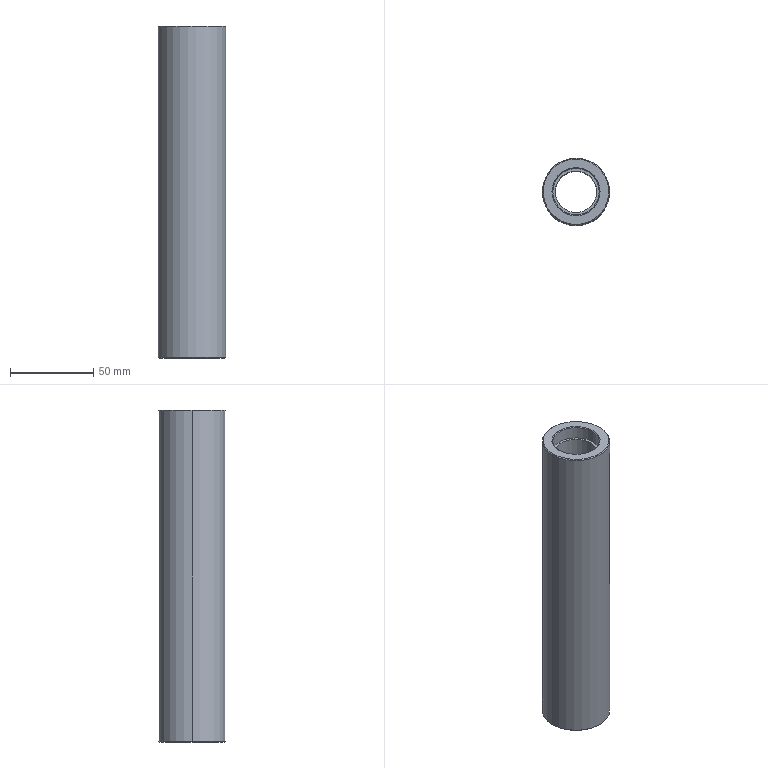Part | SolidWorks | features ICE 2, Chamfer 1, Extrusion 1, MirrorPattern 1 | 1 solid | 20 faces | box 40.5 x 40.5 x 200 mm | volume 157423 mm3 | cone 8 | cylinder 8 | plane 4 | commonest cylinder face diameters 28 x4 25 x2 40.5 x2
STEP:
#1=CARTESIAN_POINT('',(19.75,0.,100.));
#2=VERTEX_POINT('',#1);
#3=CARTESIAN_POINT('',(-19.75,0.,100.));
#4=VERTEX_POINT('',#3);
#5=CARTESIAN_POINT('',(0.,0.,100.));
#6=DIRECTION('',(0.,0.,1.));
#7=DIRECTION('',(1.,0.,0.));
#8=AXIS2_PLACEMENT_3D('',#5,#6,#7);
#9=CIRCLE('',#8,19.75);
#10=EDGE_CURVE('',#2,#4,#9,.T.);
#11=ORIENTED_EDGE('',*,*,#10,.F.);
#12=CARTESIAN_POINT('',(20.25,0.,99.5));
#13=VERTEX_POINT('',#12);
#14=CARTESIAN_POINT('',(19.75,0.,100.));
#15=DIRECTION('',(0.7071,0.,-0.7071));
#16=VECTOR('',#15,1000.);
#17=LINE('',#14,#16);
#18=EDGE_CURVE('',#2,#13,#17,.T.);
#19=ORIENTED_EDGE('',*,*,#18,.T.);
#20=CARTESIAN_POINT('',(-20.25,0.,99.5));
#21=VERTEX_POINT('',#20);
#22=CARTESIAN_POINT('',(0.,0.,99.5));
#23=DIRECTION('',(0.,0.,-1.));
#24=DIRECTION('',(1.,0.,0.));
#25=AXIS2_PLACEMENT_3D('',#22,#23,#24);
#26=CIRCLE('',#25,20.25);
#27=EDGE_CURVE('',#21,#13,#26,.T.);
#28=ORIENTED_EDGE('',*,*,#27,.F.);
#29=CARTESIAN_POINT('',(-19.75,0.,100.));
#30=DIRECTION('',(-0.7071,0.,-0.7071));
#31=VECTOR('',#30,1000.);
#32=LINE('',#29,#31);
#33=EDGE_CURVE('',#4,#21,#32,.T.);
#34=ORIENTED_EDGE('',*,*,#33,.F.);
#35=EDGE_LOOP('',(#11,#19,#28,#34));
#36=FACE_OUTER_BOUND('',#35,.T.);
#37=CARTESIAN_POINT('',(0.,0.,100.));
#38=DIRECTION('',(0.,0.,-1.));
#39=DIRECTION('',(-1.,0.,0.));
#40=AXIS2_PLACEMENT_3D('',#37,#38,#39);
#41=CONICAL_SURFACE('',#40,19.75,0.7854);
#42=ADVANCED_FACE('',(#36),#41,.T.);
#43=CARTESIAN_POINT('',(-19.75,0.,-100.));
#44=VERTEX_POINT('',#43);
#45=CARTESIAN_POINT('',(19.75,0.,-100.));
#46=VERTEX_POINT('',#45);
#47=CARTESIAN_POINT('',(0.,0.,-100.));
#48=DIRECTION('',(0.,0.,-1.));
#49=DIRECTION('',(1.,0.,0.));
#50=AXIS2_PLACEMENT_3D('',#47,#48,#49);
#51=CIRCLE('',#50,19.75);
#52=EDGE_CURVE('',#44,#46,#51,.T.);
#53=ORIENTED_EDGE('',*,*,#52,.F.);
#54=CARTESIAN_POINT('',(-20.25,0.,-99.5));
#55=VERTEX_POINT('',#54);
#56=CARTESIAN_POINT('',(-20.25,0.,-99.5));
#57=DIRECTION('',(-0.7071,0.,0.7071));
#58=VECTOR('',#57,1000.);
#59=LINE('',#56,#58);
#60=EDGE_CURVE('',#44,#55,#59,.T.);
#61=ORIENTED_EDGE('',*,*,#60,.T.);
#62=CARTESIAN_POINT('',(20.25,0.,-99.5));
#63=VERTEX_POINT('',#62);
#64=CARTESIAN_POINT('',(0.,0.,-99.5));
#65=DIRECTION('',(0.,0.,1.));
#66=DIRECTION('',(1.,0.,0.));
#67=AXIS2_PLACEMENT_3D('',#64,#65,#66);
#68=CIRCLE('',#67,20.25);
#69=EDGE_CURVE('',#63,#55,#68,.T.);
#70=ORIENTED_EDGE('',*,*,#69,.F.);
#71=CARTESIAN_POINT('',(20.25,0.,-99.5));
#72=DIRECTION('',(0.7071,0.,0.7071));
#73=VECTOR('',#72,1000.);
#74=LINE('',#71,#73);
#75=EDGE_CURVE('',#46,#63,#74,.T.);
#76=ORIENTED_EDGE('',*,*,#75,.F.);
#77=EDGE_LOOP('',(#53,#61,#70,#76));
#78=FACE_OUTER_BOUND('',#77,.T.);
#79=CARTESIAN_POINT('',(0.,0.,-99.5));
#80=DIRECTION('',(0.,0.,1.));
#81=DIRECTION('',(1.,0.,0.));
#82=AXIS2_PLACEMENT_3D('',#79,#80,#81);
#83=CONICAL_SURFACE('',#82,20.25,0.7854);
#84=ADVANCED_FACE('',(#78),#83,.T.);
#85=CARTESIAN_POINT('',(14.,0.,-99.5));
#86=VERTEX_POINT('',#85);
#87=CARTESIAN_POINT('',(-14.,0.,-99.5));
#88=VERTEX_POINT('',#87);
#89=CARTESIAN_POINT('',(0.,0.,-99.5));
#90=DIRECTION('',(0.,0.,-1.));
#91=DIRECTION('',(1.,0.,0.));
#92=AXIS2_PLACEMENT_3D('',#89,#90,#91);
#93=CIRCLE('',#92,14.);
#94=EDGE_CURVE('',#86,#88,#93,.T.);
#95=ORIENTED_EDGE('',*,*,#94,.F.);
#96=CARTESIAN_POINT('',(14.5,0.,-100.));
#97=VERTEX_POINT('',#96);
#98=CARTESIAN_POINT('',(14.5,0.,-100.));
#99=DIRECTION('',(0.7071,0.,-0.7071));
#100=VECTOR('',#99,1000.);
#101=LINE('',#98,#100);
#102=EDGE_CURVE('',#86,#97,#101,.T.);
#103=ORIENTED_EDGE('',*,*,#102,.T.);
#104=CARTESIAN_POINT('',(-14.5,0.,-100.));
#105=VERTEX_POINT('',#104);
#106=CARTESIAN_POINT('',(0.,0.,-100.));
#107=DIRECTION('',(0.,0.,1.));
#108=DIRECTION('',(1.,0.,0.));
#109=AXIS2_PLACEMENT_3D('',#106,#107,#108);
#110=CIRCLE('',#109,14.5);
#111=EDGE_CURVE('',#105,#97,#110,.T.);
#112=ORIENTED_EDGE('',*,*,#111,.F.);
#113=CARTESIAN_POINT('',(-14.5,0.,-100.));
#114=DIRECTION('',(-0.7071,0.,-0.7071));
#115=VECTOR('',#114,1000.);
#116=LINE('',#113,#115);
#117=EDGE_CURVE('',#88,#105,#116,.T.);
#118=ORIENTED_EDGE('',*,*,#117,.F.);
#119=EDGE_LOOP('',(#95,#103,#112,#118));
#120=FACE_OUTER_BOUND('',#119,.T.);
#121=CARTESIAN_POINT('',(0.,0.,-100.));
#122=DIRECTION('',(0.,0.,-1.));
#123=DIRECTION('',(-1.,0.,0.));
#124=AXIS2_PLACEMENT_3D('',#121,#122,#123);
#125=CONICAL_SURFACE('',#124,14.5,0.7854);
#126=ADVANCED_FACE('',(#120),#125,.F.);
#127=CARTESIAN_POINT('',(-14.,0.,99.5));
#128=VERTEX_POINT('',#127);
#129=CARTESIAN_POINT('',(14.,0.,99.5));
#130=VERTEX_POINT('',#129);
#131=CARTESIAN_POINT('',(0.,0.,99.5));
#132=DIRECTION('',(0.,0.,1.));
#133=DIRECTION('',(1.,0.,0.));
#134=AXIS2_PLACEMENT_3D('',#131,#132,#133);
#135=CIRCLE('',#134,14.);
#136=EDGE_CURVE('',#128,#130,#135,.T.);
#137=ORIENTED_EDGE('',*,*,#136,.F.);
#138=CARTESIAN_POINT('',(-14.5,0.,100.));
#139=VERTEX_POINT('',#138);
#140=CARTESIAN_POINT('',(-14.,0.,99.5));
#141=DIRECTION('',(-0.7071,0.,0.7071));
#142=VECTOR('',#141,1000.);
#143=LINE('',#140,#142);
#144=EDGE_CURVE('',#128,#139,#143,.T.);
#145=ORIENTED_EDGE('',*,*,#144,.T.);
#146=CARTESIAN_POINT('',(14.5,0.,100.));
#147=VERTEX_POINT('',#146);
#148=CARTESIAN_POINT('',(0.,0.,100.));
#149=DIRECTION('',(0.,0.,-1.));
#150=DIRECTION('',(1.,0.,0.));
#151=AXIS2_PLACEMENT_3D('',#148,#149,#150);
#152=CIRCLE('',#151,14.5);
#153=EDGE_CURVE('',#147,#139,#152,.T.);
#154=ORIENTED_EDGE('',*,*,#153,.F.);
#155=CARTESIAN_POINT('',(14.,0.,99.5));
#156=DIRECTION('',(0.7071,0.,0.7071));
#157=VECTOR('',#156,1000.);
#158=LINE('',#155,#157);
#159=EDGE_CURVE('',#130,#147,#158,.T.);
#160=ORIENTED_EDGE('',*,*,#159,.F.);
#161=EDGE_LOOP('',(#137,#145,#154,#160));
#162=FACE_OUTER_BOUND('',#161,.T.);
#163=CARTESIAN_POINT('',(0.,0.,99.5));
#164=DIRECTION('',(0.,0.,1.));
#165=DIRECTION('',(1.,0.,0.));
#166=AXIS2_PLACEMENT_3D('',#163,#164,#165);
#167=CONICAL_SURFACE('',#166,14.,0.7854);
#168=ADVANCED_FACE('',(#162),#167,.F.);
#169=CARTESIAN_POINT('',(12.5,0.,-92.));
#170=VERTEX_POINT('',#169);
#171=CARTESIAN_POINT('',(-12.5,0.,-92.));
#172=VERTEX_POINT('',#171);
#173=CARTESIAN_POINT('',(0.,0.,-92.));
#174=DIRECTION('',(0.,0.,-1.));
#175=DIRECTION('',(-1.,0.,0.));
#176=AXIS2_PLACEMENT_3D('',#173,#174,#175);
#177=CIRCLE('',#176,12.5);
#178=EDGE_CURVE('',#170,#172,#177,.T.);
#179=ORIENTED_EDGE('',*,*,#178,.T.);
#180=CARTESIAN_POINT('',(-12.5,0.,92.));
#181=VERTEX_POINT('',#180);
#182=CARTESIAN_POINT('',(-12.5,0.,-100.));
#183=DIRECTION('',(0.,0.,1.));
#184=VECTOR('',#183,1000.);
#185=LINE('',#182,#184);
#186=EDGE_CURVE('',#172,#181,#185,.T.);
#187=ORIENTED_EDGE('',*,*,#186,.T.);
#188=CARTESIAN_POINT('',(12.5,0.,92.));
#189=VERTEX_POINT('',#188);
#190=CARTESIAN_POINT('',(0.,0.,92.));
#191=DIRECTION('',(0.,0.,1.));
#192=DIRECTION('',(1.,0.,0.));
#193=AXIS2_PLACEMENT_3D('',#190,#191,#192);
#194=CIRCLE('',#193,12.5);
#195=EDGE_CURVE('',#181,#189,#194,.T.);
#196=ORIENTED_EDGE('',*,*,#195,.T.);
#197=CARTESIAN_POINT('',(12.5,0.,-100.));
#198=DIRECTION('',(0.,0.,1.));
#199=VECTOR('',#198,1000.);
#200=LINE('',#197,#199);
#201=EDGE_CURVE('',#170,#189,#200,.T.);
#202=ORIENTED_EDGE('',*,*,#201,.F.);
#203=EDGE_LOOP('',(#179,#187,#196,#202));
#204=FACE_OUTER_BOUND('',#203,.T.);
#205=CARTESIAN_POINT('',(0.,0.,-100.));
#206=DIRECTION('',(0.,0.,1.));
#207=DIRECTION('',(1.,0.,0.));
#208=AXIS2_PLACEMENT_3D('',#205,#206,#207);
#209=CYLINDRICAL_SURFACE('',#208,12.5);
#210=ADVANCED_FACE('',(#204),#209,.F.);
#211=CARTESIAN_POINT('',(-14.,0.,-92.));
#212=VERTEX_POINT('',#211);
#213=CARTESIAN_POINT('',(14.,0.,-92.));
#214=VERTEX_POINT('',#213);
#215=CARTESIAN_POINT('',(0.,0.,-92.));
#216=DIRECTION('',(0.,0.,1.));
#217=DIRECTION('',(1.,0.,0.));
#218=AXIS2_PLACEMENT_3D('',#215,#216,#217);
#219=CIRCLE('',#218,14.);
#220=EDGE_CURVE('',#212,#214,#219,.T.);
#221=ORIENTED_EDGE('',*,*,#220,.T.);
#222=CARTESIAN_POINT('',(14.,0.,-92.));
#223=DIRECTION('',(0.,0.,-1.));
#224=VECTOR('',#223,1000.);
#225=LINE('',#222,#224);
#226=EDGE_CURVE('',#214,#86,#225,.T.);
#227=ORIENTED_EDGE('',*,*,#226,.T.);
#228=ORIENTED_EDGE('',*,*,#94,.T.);
#229=CARTESIAN_POINT('',(-14.,0.,-92.));
#230=DIRECTION('',(0.,0.,-1.));
#231=VECTOR('',#230,1000.);
#232=LINE('',#229,#231);
#233=EDGE_CURVE('',#212,#88,#232,.T.);
#234=ORIENTED_EDGE('',*,*,#233,.F.);
#235=EDGE_LOOP('',(#221,#227,#228,#234));
#236=FACE_OUTER_BOUND('',#235,.T.);
#237=CARTESIAN_POINT('',(0.,0.,-92.));
#238=DIRECTION('',(0.,0.,-1.));
#239=DIRECTION('',(-1.,0.,0.));
#240=AXIS2_PLACEMENT_3D('',#237,#238,#239);
#241=CYLINDRICAL_SURFACE('',#240,14.);
#242=ADVANCED_FACE('',(#236),#241,.F.);
#243=CARTESIAN_POINT('',(-14.,0.,92.));
#244=VERTEX_POINT('',#243);
#245=CARTESIAN_POINT('',(14.,0.,92.));
#246=VERTEX_POINT('',#245);
#247=CARTESIAN_POINT('',(0.,0.,92.));
#248=DIRECTION('',(0.,0.,1.));
#249=DIRECTION('',(1.,0.,0.));
#250=AXIS2_PLACEMENT_3D('',#247,#248,#249);
#251=CIRCLE('',#250,14.);
#252=EDGE_CURVE('',#244,#246,#251,.T.);
#253=ORIENTED_EDGE('',*,*,#252,.F.);
#254=CARTESIAN_POINT('',(-14.,0.,92.));
#255=DIRECTION('',(0.,0.,1.));
#256=VECTOR('',#255,1000.);
#257=LINE('',#254,#256);
#258=EDGE_CURVE('',#244,#128,#257,.T.);
#259=ORIENTED_EDGE('',*,*,#258,.T.);
#260=ORIENTED_EDGE('',*,*,#136,.T.);
#261=CARTESIAN_POINT('',(14.,0.,92.));
#262=DIRECTION('',(0.,0.,1.));
#263=VECTOR('',#262,1000.);
#264=LINE('',#261,#263);
#265=EDGE_CURVE('',#246,#130,#264,.T.);
#266=ORIENTED_EDGE('',*,*,#265,.F.);
#267=EDGE_LOOP('',(#253,#259,#260,#266));
#268=FACE_OUTER_BOUND('',#267,.T.);
#269=CARTESIAN_POINT('',(0.,0.,92.));
#270=DIRECTION('',(0.,0.,1.));
#271=DIRECTION('',(1.,0.,0.));
#272=AXIS2_PLACEMENT_3D('',#269,#270,#271);
#273=CYLINDRICAL_SURFACE('',#272,14.);
#274=ADVANCED_FACE('',(#268),#273,.F.);
#275=ORIENTED_EDGE('',*,*,#27,.T.);
#276=CARTESIAN_POINT('',(20.25,0.,100.));
#277=DIRECTION('',(0.,0.,-1.));
#278=VECTOR('',#277,1000.);
#279=LINE('',#276,#278);
#280=EDGE_CURVE('',#13,#63,#279,.T.);
#281=ORIENTED_EDGE('',*,*,#280,.T.);
#282=ORIENTED_EDGE('',*,*,#69,.T.);
#283=CARTESIAN_POINT('',(-20.25,0.,100.));
#284=DIRECTION('',(0.,0.,-1.));
#285=VECTOR('',#284,1000.);
#286=LINE('',#283,#285);
#287=EDGE_CURVE('',#21,#55,#286,.T.);
#288=ORIENTED_EDGE('',*,*,#287,.F.);
#289=EDGE_LOOP('',(#275,#281,#282,#288));
#290=FACE_OUTER_BOUND('',#289,.T.);
#291=CARTESIAN_POINT('',(0.,0.,100.));
#292=DIRECTION('',(0.,0.,-1.));
#293=DIRECTION('',(-1.,0.,0.));
#294=AXIS2_PLACEMENT_3D('',#291,#292,#293);
#295=CYLINDRICAL_SURFACE('',#294,20.25);
#296=ADVANCED_FACE('',(#290),#295,.T.);
#297=ORIENTED_EDGE('',*,*,#280,.F.);
#298=CARTESIAN_POINT('',(0.,0.,99.5));
#299=DIRECTION('',(0.,0.,-1.));
#300=DIRECTION('',(1.,0.,0.));
#301=AXIS2_PLACEMENT_3D('',#298,#299,#300);
#302=CIRCLE('',#301,20.25);
#303=EDGE_CURVE('',#13,#21,#302,.T.);
#304=ORIENTED_EDGE('',*,*,#303,.T.);
#305=ORIENTED_EDGE('',*,*,#287,.T.);
#306=CARTESIAN_POINT('',(0.,0.,-99.5));
#307=DIRECTION('',(0.,0.,1.));
#308=DIRECTION('',(1.,0.,0.));
#309=AXIS2_PLACEMENT_3D('',#306,#307,#308);
#310=CIRCLE('',#309,20.25);
#311=EDGE_CURVE('',#55,#63,#310,.T.);
#312=ORIENTED_EDGE('',*,*,#311,.T.);
#313=EDGE_LOOP('',(#297,#304,#305,#312));
#314=FACE_OUTER_BOUND('',#313,.T.);
#315=CARTESIAN_POINT('',(0.,0.,100.));
#316=DIRECTION('',(0.,0.,-1.));
#317=DIRECTION('',(-1.,0.,0.));
#318=AXIS2_PLACEMENT_3D('',#315,#316,#317);
#319=CYLINDRICAL_SURFACE('',#318,20.25);
#320=ADVANCED_FACE('',(#314),#319,.T.);
#321=ORIENTED_EDGE('',*,*,#153,.T.);
#322=CARTESIAN_POINT('',(0.,0.,100.));
#323=DIRECTION('',(0.,0.,-1.));
#324=DIRECTION('',(1.,0.,0.));
#325=AXIS2_PLACEMENT_3D('',#322,#323,#324);
#326=CIRCLE('',#325,14.5);
#327=EDGE_CURVE('',#139,#147,#326,.T.);
#328=ORIENTED_EDGE('',*,*,#327,.T.);
#329=EDGE_LOOP('',(#321,#328));
#330=FACE_BOUND('',#329,.T.);
#331=CARTESIAN_POINT('',(0.,0.,100.));
#332=DIRECTION('',(0.,0.,1.));
#333=DIRECTION('',(1.,0.,0.));
#334=AXIS2_PLACEMENT_3D('',#331,#332,#333);
#335=CIRCLE('',#334,19.75);
#336=EDGE_CURVE('',#4,#2,#335,.T.);
#337=ORIENTED_EDGE('',*,*,#336,.T.);
#338=ORIENTED_EDGE('',*,*,#10,.T.);
#339=EDGE_LOOP('',(#337,#338));
#340=FACE_OUTER_BOUND('',#339,.T.);
#341=CARTESIAN_POINT('',(0.,0.,100.));
#342=DIRECTION('',(0.,0.,1.));
#343=DIRECTION('',(1.,0.,0.));
#344=AXIS2_PLACEMENT_3D('',#341,#342,#343);
#345=PLANE('',#344);
#346=ADVANCED_FACE('',(#330,#340),#345,.T.);
#347=ORIENTED_EDGE('',*,*,#111,.T.);
#348=CARTESIAN_POINT('',(0.,0.,-100.));
#349=DIRECTION('',(0.,0.,1.));
#350=DIRECTION('',(1.,0.,0.));
#351=AXIS2_PLACEMENT_3D('',#348,#349,#350);
#352=CIRCLE('',#351,14.5);
#353=EDGE_CURVE('',#97,#105,#352,.T.);
#354=ORIENTED_EDGE('',*,*,#353,.T.);
#355=EDGE_LOOP('',(#347,#354));
#356=FACE_BOUND('',#355,.T.);
#357=CARTESIAN_POINT('',(0.,0.,-100.));
#358=DIRECTION('',(0.,0.,-1.));
#359=DIRECTION('',(1.,0.,0.));
#360=AXIS2_PLACEMENT_3D('',#357,#358,#359);
#361=CIRCLE('',#360,19.75);
#362=EDGE_CURVE('',#46,#44,#361,.T.);
#363=ORIENTED_EDGE('',*,*,#362,.T.);
#364=ORIENTED_EDGE('',*,*,#52,.T.);
#365=EDGE_LOOP('',(#363,#364));
#366=FACE_OUTER_BOUND('',#365,.T.);
#367=CARTESIAN_POINT('',(0.,0.,-100.));
#368=DIRECTION('',(0.,0.,1.));
#369=DIRECTION('',(1.,0.,0.));
#370=AXIS2_PLACEMENT_3D('',#367,#368,#369);
#371=PLANE('',#370);
#372=ADVANCED_FACE('',(#356,#366),#371,.F.);
#373=ORIENTED_EDGE('',*,*,#258,.F.);
#374=CARTESIAN_POINT('',(0.,0.,92.));
#375=DIRECTION('',(0.,0.,1.));
#376=DIRECTION('',(1.,0.,0.));
#377=AXIS2_PLACEMENT_3D('',#374,#375,#376);
#378=CIRCLE('',#377,14.);
#379=EDGE_CURVE('',#246,#244,#378,.T.);
#380=ORIENTED_EDGE('',*,*,#379,.F.);
#381=ORIENTED_EDGE('',*,*,#265,.T.);
#382=CARTESIAN_POINT('',(0.,0.,99.5));
#383=DIRECTION('',(0.,0.,1.));
#384=DIRECTION('',(1.,0.,0.));
#385=AXIS2_PLACEMENT_3D('',#382,#383,#384);
#386=CIRCLE('',#385,14.);
#387=EDGE_CURVE('',#130,#128,#386,.T.);
#388=ORIENTED_EDGE('',*,*,#387,.T.);
#389=EDGE_LOOP('',(#373,#380,#381,#388));
#390=FACE_OUTER_BOUND('',#389,.T.);
#391=CARTESIAN_POINT('',(0.,0.,92.));
#392=DIRECTION('',(0.,0.,1.));
#393=DIRECTION('',(1.,0.,0.));
#394=AXIS2_PLACEMENT_3D('',#391,#392,#393);
#395=CYLINDRICAL_SURFACE('',#394,14.);
#396=ADVANCED_FACE('',(#390),#395,.F.);
#397=CARTESIAN_POINT('',(0.,0.,92.));
#398=DIRECTION('',(0.,0.,1.));
#399=DIRECTION('',(1.,0.,0.));
#400=AXIS2_PLACEMENT_3D('',#397,#398,#399);
#401=CIRCLE('',#400,12.5);
#402=EDGE_CURVE('',#189,#181,#401,.T.);
#403=ORIENTED_EDGE('',*,*,#402,.F.);
#404=ORIENTED_EDGE('',*,*,#195,.F.);
#405=EDGE_LOOP('',(#403,#404));
#406=FACE_BOUND('',#405,.T.);
#407=ORIENTED_EDGE('',*,*,#379,.T.);
#408=ORIENTED_EDGE('',*,*,#252,.T.);
#409=EDGE_LOOP('',(#407,#408));
#410=FACE_OUTER_BOUND('',#409,.T.);
#411=CARTESIAN_POINT('',(0.,0.,92.));
#412=DIRECTION('',(0.,0.,1.));
#413=DIRECTION('',(1.,0.,0.));
#414=AXIS2_PLACEMENT_3D('',#411,#412,#413);
#415=PLANE('',#414);
#416=ADVANCED_FACE('',(#406,#410),#415,.T.);
#417=ORIENTED_EDGE('',*,*,#226,.F.);
#418=CARTESIAN_POINT('',(0.,0.,-92.));
#419=DIRECTION('',(0.,0.,1.));
#420=DIRECTION('',(1.,0.,0.));
#421=AXIS2_PLACEMENT_3D('',#418,#419,#420);
#422=CIRCLE('',#421,14.);
#423=EDGE_CURVE('',#214,#212,#422,.T.);
#424=ORIENTED_EDGE('',*,*,#423,.T.);
#425=ORIENTED_EDGE('',*,*,#233,.T.);
#426=CARTESIAN_POINT('',(0.,0.,-99.5));
#427=DIRECTION('',(0.,0.,-1.));
#428=DIRECTION('',(1.,0.,0.));
#429=AXIS2_PLACEMENT_3D('',#426,#427,#428);
#430=CIRCLE('',#429,14.);
#431=EDGE_CURVE('',#88,#86,#430,.T.);
#432=ORIENTED_EDGE('',*,*,#431,.T.);
#433=EDGE_LOOP('',(#417,#424,#425,#432));
#434=FACE_OUTER_BOUND('',#433,.T.);
#435=CARTESIAN_POINT('',(0.,0.,-92.));
#436=DIRECTION('',(0.,0.,-1.));
#437=DIRECTION('',(-1.,0.,0.));
#438=AXIS2_PLACEMENT_3D('',#435,#436,#437);
#439=CYLINDRICAL_SURFACE('',#438,14.);
#440=ADVANCED_FACE('',(#434),#439,.F.);
#441=ORIENTED_EDGE('',*,*,#178,.F.);
#442=CARTESIAN_POINT('',(0.,0.,-92.));
#443=DIRECTION('',(0.,0.,-1.));
#444=DIRECTION('',(-1.,0.,0.));
#445=AXIS2_PLACEMENT_3D('',#442,#443,#444);
#446=CIRCLE('',#445,12.5);
#447=EDGE_CURVE('',#172,#170,#446,.T.);
#448=ORIENTED_EDGE('',*,*,#447,.F.);
#449=EDGE_LOOP('',(#441,#448));
#450=FACE_BOUND('',#449,.T.);
#451=ORIENTED_EDGE('',*,*,#220,.F.);
#452=ORIENTED_EDGE('',*,*,#423,.F.);
#453=EDGE_LOOP('',(#451,#452));
#454=FACE_OUTER_BOUND('',#453,.T.);
#455=CARTESIAN_POINT('',(0.,0.,-92.));
#456=DIRECTION('',(0.,0.,-1.));
#457=DIRECTION('',(1.,0.,0.));
#458=AXIS2_PLACEMENT_3D('',#455,#456,#457);
#459=PLANE('',#458);
#460=ADVANCED_FACE('',(#450,#454),#459,.T.);
#461=ORIENTED_EDGE('',*,*,#186,.F.);
#462=ORIENTED_EDGE('',*,*,#447,.T.);
#463=ORIENTED_EDGE('',*,*,#201,.T.);
#464=ORIENTED_EDGE('',*,*,#402,.T.);
#465=EDGE_LOOP('',(#461,#462,#463,#464));
#466=FACE_OUTER_BOUND('',#465,.T.);
#467=CARTESIAN_POINT('',(0.,0.,-100.));
#468=DIRECTION('',(0.,0.,1.));
#469=DIRECTION('',(1.,0.,0.));
#470=AXIS2_PLACEMENT_3D('',#467,#468,#469);
#471=CYLINDRICAL_SURFACE('',#470,12.5);
#472=ADVANCED_FACE('',(#466),#471,.F.);
#473=ORIENTED_EDGE('',*,*,#144,.F.);
#474=ORIENTED_EDGE('',*,*,#387,.F.);
#475=ORIENTED_EDGE('',*,*,#159,.T.);
#476=ORIENTED_EDGE('',*,*,#327,.F.);
#477=EDGE_LOOP('',(#473,#474,#475,#476));
#478=FACE_OUTER_BOUND('',#477,.T.);
#479=CARTESIAN_POINT('',(0.,0.,99.5));
#480=DIRECTION('',(0.,0.,1.));
#481=DIRECTION('',(1.,0.,0.));
#482=AXIS2_PLACEMENT_3D('',#479,#480,#481);
#483=CONICAL_SURFACE('',#482,14.,0.7854);
#484=ADVANCED_FACE('',(#478),#483,.F.);
#485=ORIENTED_EDGE('',*,*,#102,.F.);
#486=ORIENTED_EDGE('',*,*,#431,.F.);
#487=ORIENTED_EDGE('',*,*,#117,.T.);
#488=ORIENTED_EDGE('',*,*,#353,.F.);
#489=EDGE_LOOP('',(#485,#486,#487,#488));
#490=FACE_OUTER_BOUND('',#489,.T.);
#491=CARTESIAN_POINT('',(0.,0.,-100.));
#492=DIRECTION('',(0.,0.,-1.));
#493=DIRECTION('',(-1.,0.,0.));
#494=AXIS2_PLACEMENT_3D('',#491,#492,#493);
#495=CONICAL_SURFACE('',#494,14.5,0.7854);
#496=ADVANCED_FACE('',(#490),#495,.F.);
#497=ORIENTED_EDGE('',*,*,#60,.F.);
#498=ORIENTED_EDGE('',*,*,#362,.F.);
#499=ORIENTED_EDGE('',*,*,#75,.T.);
#500=ORIENTED_EDGE('',*,*,#311,.F.);
#501=EDGE_LOOP('',(#497,#498,#499,#500));
#502=FACE_OUTER_BOUND('',#501,.T.);
#503=CARTESIAN_POINT('',(0.,0.,-99.5));
#504=DIRECTION('',(0.,0.,1.));
#505=DIRECTION('',(1.,0.,0.));
#506=AXIS2_PLACEMENT_3D('',#503,#504,#505);
#507=CONICAL_SURFACE('',#506,20.25,0.7854);
#508=ADVANCED_FACE('',(#502),#507,.T.);
#509=ORIENTED_EDGE('',*,*,#18,.F.);
#510=ORIENTED_EDGE('',*,*,#336,.F.);
#511=ORIENTED_EDGE('',*,*,#33,.T.);
#512=ORIENTED_EDGE('',*,*,#303,.F.);
#513=EDGE_LOOP('',(#509,#510,#511,#512));
#514=FACE_OUTER_BOUND('',#513,.T.);
#515=CARTESIAN_POINT('',(0.,0.,100.));
#516=DIRECTION('',(0.,0.,-1.));
#517=DIRECTION('',(-1.,0.,0.));
#518=AXIS2_PLACEMENT_3D('',#515,#516,#517);
#519=CONICAL_SURFACE('',#518,19.75,0.7854);
#520=ADVANCED_FACE('',(#514),#519,.T.);
#521=CLOSED_SHELL('',(#42,#84,#126,#168,#210,#242,#274,#296,#320,#346,#372,#396,#416,#440,#460,#472,#484,#496,#508,#520));
#522=MANIFOLD_SOLID_BREP('',#521);
#523=CARTESIAN_POINT('',(0.,0.,0.));
#524=DIRECTION('',(0.,0.,1.));
#525=DIRECTION('',(1.,0.,0.));
#526=AXIS2_PLACEMENT_3D('',#523,#524,#525);
#527=(LENGTH_UNIT()NAMED_UNIT(*)SI_UNIT(.MILLI.,.METRE.));
#528=UNCERTAINTY_MEASURE_WITH_UNIT(LENGTH_MEASURE(0.00001),#527,'','');
#529=(NAMED_UNIT(*)PLANE_ANGLE_UNIT()SI_UNIT($,.RADIAN.));
#530=(NAMED_UNIT(*)SI_UNIT($,.STERADIAN.)SOLID_ANGLE_UNIT());
#531=(GEOMETRIC_REPRESENTATION_CONTEXT(3)GLOBAL_UNCERTAINTY_ASSIGNED_CONTEXT((#528))GLOBAL_UNIT_ASSIGNED_CONTEXT((#527,#529,#530))REPRESENTATION_CONTEXT('',''));
#532=ADVANCED_BREP_SHAPE_REPRESENTATION('',(#522,#526),#531);